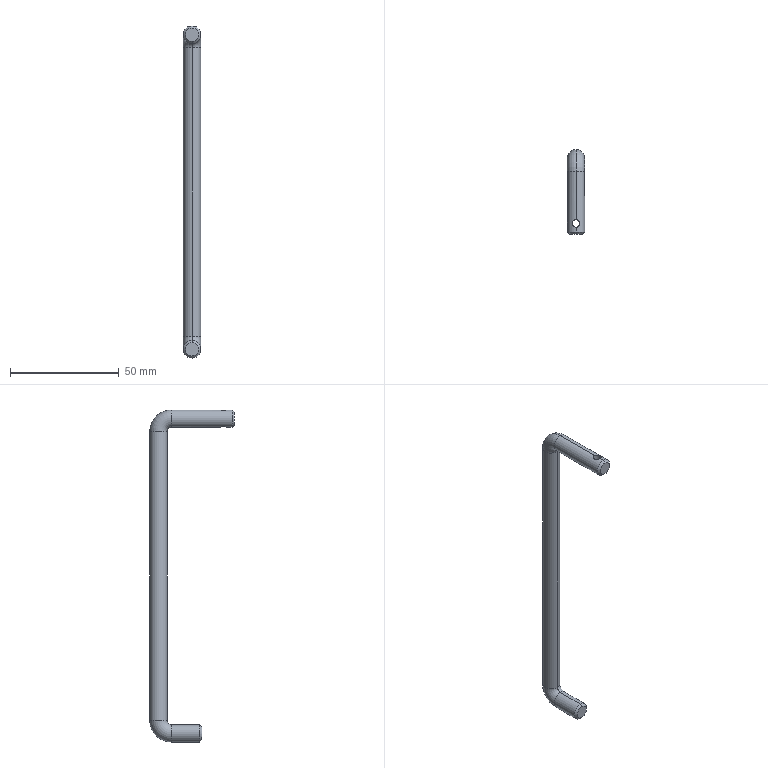Part | SolidWorks | features BaseBody 1 | 1 solid | 18 faces | box 8 x 39 x 153 mm | volume 9696 mm3 | cylinder 8 | cone 4 | torus 4 | plane 2 | commonest cylinder face diameters 8 x6 3.5 x2
STEP:
#1=CARTESIAN_POINT('',(1.75,-30.,76.097));
#2=VERTEX_POINT('',#1);
#3=CARTESIAN_POINT('',(1.75,-30.,68.903));
#4=VERTEX_POINT('',#3);
#5=CARTESIAN_POINT('',(1.75,-30.,132.));
#6=DIRECTION('',(0.,0.,-1.));
#7=VECTOR('',#6,1000.);
#8=LINE('',#5,#7);
#9=EDGE_CURVE('',#2,#4,#8,.T.);
#10=ORIENTED_EDGE('',*,*,#9,.F.);
#11=CARTESIAN_POINT('',(0.,-28.25,76.5));
#12=VERTEX_POINT('',#11);
#13=CARTESIAN_POINT('',(0.,-28.25,76.5));
#14=CARTESIAN_POINT('',(0.1167,-28.25,76.5));
#15=CARTESIAN_POINT('',(0.2317,-28.261,76.495));
#16=CARTESIAN_POINT('',(0.4573,-28.307,76.475));
#17=CARTESIAN_POINT('',(0.5697,-28.341,76.461));
#18=CARTESIAN_POINT('',(0.8889,-28.475,76.406));
#19=CARTESIAN_POINT('',(1.075,-28.6,76.357));
#20=CARTESIAN_POINT('',(1.321,-28.847,76.276));
#21=CARTESIAN_POINT('',(1.393,-28.935,76.25));
#22=CARTESIAN_POINT('',(1.487,-29.075,76.213));
#23=CARTESIAN_POINT('',(1.516,-29.124,76.202));
#24=CARTESIAN_POINT('',(1.569,-29.223,76.179));
#25=CARTESIAN_POINT('',(1.593,-29.272,76.169));
#26=CARTESIAN_POINT('',(1.706,-29.544,76.119));
#27=CARTESIAN_POINT('',(1.75,-29.768,76.097));
#28=CARTESIAN_POINT('',(1.75,-30.,76.097));
#29=B_SPLINE_CURVE_WITH_KNOTS('',3,(#13,#14,#15,#16,#17,#18,#19,#20,#21,#22,#23,#24,#25,#26,#27,#28),.UNSPECIFIED.,.F.,.F.,(4,2,2,2,2,2,2,4),(0.,0.125,0.25,0.5,0.625,0.6875,0.75,1.),.UNSPECIFIED.);
#30=EDGE_CURVE('',#12,#2,#29,.T.);
#31=ORIENTED_EDGE('',*,*,#30,.F.);
#32=CARTESIAN_POINT('',(-1.75,-30.,76.097));
#33=VERTEX_POINT('',#32);
#34=CARTESIAN_POINT('',(-1.75,-30.,76.097));
#35=CARTESIAN_POINT('',(-1.75,-29.884,76.097));
#36=CARTESIAN_POINT('',(-1.739,-29.769,76.102));
#37=CARTESIAN_POINT('',(-1.705,-29.6,76.118));
#38=CARTESIAN_POINT('',(-1.691,-29.545,76.125));
#39=CARTESIAN_POINT('',(-1.666,-29.462,76.137));
#40=CARTESIAN_POINT('',(-1.656,-29.434,76.141));
#41=CARTESIAN_POINT('',(-1.636,-29.379,76.15));
#42=CARTESIAN_POINT('',(-1.625,-29.351,76.155));
#43=CARTESIAN_POINT('',(-1.571,-29.22,76.179));
#44=CARTESIAN_POINT('',(-1.516,-29.118,76.202));
#45=CARTESIAN_POINT('',(-1.389,-28.93,76.252));
#46=CARTESIAN_POINT('',(-1.317,-28.842,76.278));
#47=CARTESIAN_POINT('',(-1.157,-28.683,76.33));
#48=CARTESIAN_POINT('',(-1.07,-28.611,76.355));
#49=CARTESIAN_POINT('',(-0.9274,-28.515,76.391));
#50=CARTESIAN_POINT('',(-0.8785,-28.486,76.403));
#51=CARTESIAN_POINT('',(-0.7783,-28.432,76.424));
#52=CARTESIAN_POINT('',(-0.7286,-28.408,76.433));
#53=CARTESIAN_POINT('',(-0.4588,-28.295,76.48));
#54=CARTESIAN_POINT('',(-0.233,-28.25,76.5));
#55=CARTESIAN_POINT('',(0.,-28.25,76.5));
#56=B_SPLINE_CURVE_WITH_KNOTS('',3,(#34,#35,#36,#37,#38,#39,#40,#41,#42,#43,#44,#45,#46,#47,#48,#49,#50,#51,#52,#53,#54,#55),.UNSPECIFIED.,.F.,.F.,(4,2,2,2,2,2,2,2,2,2,4),(0.,0.125,0.1875,0.2187,0.25,0.375,0.5,0.625,0.6875,0.75,1.),.UNSPECIFIED.);
#57=EDGE_CURVE('',#33,#12,#56,.T.);
#58=ORIENTED_EDGE('',*,*,#57,.F.);
#59=CARTESIAN_POINT('',(-1.75,-30.,68.903));
#60=VERTEX_POINT('',#59);
#61=CARTESIAN_POINT('',(-1.75,-30.,132.));
#62=DIRECTION('',(0.,0.,-1.));
#63=VECTOR('',#62,1000.);
#64=LINE('',#61,#63);
#65=EDGE_CURVE('',#33,#60,#64,.T.);
#66=ORIENTED_EDGE('',*,*,#65,.T.);
#67=CARTESIAN_POINT('',(0.,-28.25,68.5));
#68=VERTEX_POINT('',#67);
#69=CARTESIAN_POINT('',(0.,-28.25,68.5));
#70=CARTESIAN_POINT('',(-0.1167,-28.25,68.5));
#71=CARTESIAN_POINT('',(-0.2317,-28.261,68.505));
#72=CARTESIAN_POINT('',(-0.4008,-28.295,68.52));
#73=CARTESIAN_POINT('',(-0.4567,-28.309,68.526));
#74=CARTESIAN_POINT('',(-0.5672,-28.343,68.54));
#75=CARTESIAN_POINT('',(-0.6233,-28.364,68.549));
#76=CARTESIAN_POINT('',(-0.7812,-28.43,68.576));
#77=CARTESIAN_POINT('',(-0.8823,-28.485,68.597));
#78=CARTESIAN_POINT('',(-1.072,-28.612,68.645));
#79=CARTESIAN_POINT('',(-1.159,-28.684,68.671));
#80=CARTESIAN_POINT('',(-1.319,-28.844,68.723));
#81=CARTESIAN_POINT('',(-1.39,-28.93,68.748));
#82=CARTESIAN_POINT('',(-1.486,-29.074,68.786));
#83=CARTESIAN_POINT('',(-1.515,-29.123,68.798));
#84=CARTESIAN_POINT('',(-1.556,-29.198,68.815));
#85=CARTESIAN_POINT('',(-1.568,-29.223,68.82));
#86=CARTESIAN_POINT('',(-1.593,-29.274,68.831));
#87=CARTESIAN_POINT('',(-1.604,-29.299,68.836));
#88=CARTESIAN_POINT('',(-1.706,-29.543,68.881));
#89=CARTESIAN_POINT('',(-1.75,-29.768,68.903));
#90=CARTESIAN_POINT('',(-1.75,-30.,68.903));
#91=B_SPLINE_CURVE_WITH_KNOTS('',3,(#69,#70,#71,#72,#73,#74,#75,#76,#77,#78,#79,#80,#81,#82,#83,#84,#85,#86,#87,#88,#89,#90),.UNSPECIFIED.,.F.,.F.,(4,2,2,2,2,2,2,2,2,2,4),(0.,0.125,0.1875,0.25,0.375,0.5,0.625,0.6875,0.7187,0.75,1.),.UNSPECIFIED.);
#92=EDGE_CURVE('',#68,#60,#91,.T.);
#93=ORIENTED_EDGE('',*,*,#92,.F.);
#94=CARTESIAN_POINT('',(1.75,-30.,68.903));
#95=CARTESIAN_POINT('',(1.75,-29.77,68.903));
#96=CARTESIAN_POINT('',(1.703,-29.536,68.879));
#97=CARTESIAN_POINT('',(1.571,-29.221,68.821));
#98=CARTESIAN_POINT('',(1.518,-29.121,68.799));
#99=CARTESIAN_POINT('',(1.393,-28.934,68.75));
#100=CARTESIAN_POINT('',(1.319,-28.844,68.723));
#101=CARTESIAN_POINT('',(1.157,-28.682,68.67));
#102=CARTESIAN_POINT('',(1.069,-28.61,68.644));
#103=CARTESIAN_POINT('',(0.8816,-28.484,68.597));
#104=CARTESIAN_POINT('',(0.7831,-28.431,68.576));
#105=CARTESIAN_POINT('',(0.4592,-28.295,68.52));
#106=CARTESIAN_POINT('',(0.2331,-28.25,68.5));
#107=CARTESIAN_POINT('',(0.,-28.25,68.5));
#108=B_SPLINE_CURVE_WITH_KNOTS('',3,(#94,#95,#96,#97,#98,#99,#100,#101,#102,#103,#104,#105,#106,#107),.UNSPECIFIED.,.F.,.F.,(4,2,2,2,2,2,4),(0.,0.25,0.375,0.5,0.625,0.75,1.),.UNSPECIFIED.);
#109=EDGE_CURVE('',#4,#68,#108,.T.);
#110=ORIENTED_EDGE('',*,*,#109,.F.);
#111=EDGE_LOOP('',(#10,#31,#58,#66,#93,#110));
#112=FACE_OUTER_BOUND('',#111,.T.);
#113=CARTESIAN_POINT('',(0.,-30.,132.));
#114=DIRECTION('',(0.,0.,-1.));
#115=DIRECTION('',(-1.,0.,0.));
#116=AXIS2_PLACEMENT_3D('',#113,#114,#115);
#117=CYLINDRICAL_SURFACE('',#116,1.75);
#118=ADVANCED_FACE('',(#112),#117,.F.);
#119=CARTESIAN_POINT('',(0.,-35.,69.5));
#120=VERTEX_POINT('',#119);
#121=CARTESIAN_POINT('',(0.,-34.,68.5));
#122=VERTEX_POINT('',#121);
#123=CARTESIAN_POINT('',(0.,-35.,69.5));
#124=DIRECTION('',(0.,0.7071,-0.7071));
#125=VECTOR('',#124,1000.);
#126=LINE('',#123,#125);
#127=EDGE_CURVE('',#120,#122,#126,.T.);
#128=ORIENTED_EDGE('',*,*,#127,.F.);
#129=CARTESIAN_POINT('',(0.,-35.,75.5));
#130=VERTEX_POINT('',#129);
#131=CARTESIAN_POINT('',(0.,-35.,72.5));
#132=DIRECTION('',(0.,-1.,0.));
#133=DIRECTION('',(0.,0.,-1.));
#134=AXIS2_PLACEMENT_3D('',#131,#132,#133);
#135=CIRCLE('',#134,3.);
#136=EDGE_CURVE('',#130,#120,#135,.T.);
#137=ORIENTED_EDGE('',*,*,#136,.F.);
#138=CARTESIAN_POINT('',(0.,-34.,76.5));
#139=VERTEX_POINT('',#138);
#140=CARTESIAN_POINT('',(0.,-35.,75.5));
#141=DIRECTION('',(0.,0.7071,0.7071));
#142=VECTOR('',#141,1000.);
#143=LINE('',#140,#142);
#144=EDGE_CURVE('',#130,#139,#143,.T.);
#145=ORIENTED_EDGE('',*,*,#144,.T.);
#146=CARTESIAN_POINT('',(0.,-34.,72.5));
#147=DIRECTION('',(0.,1.,0.));
#148=DIRECTION('',(0.,0.,-1.));
#149=AXIS2_PLACEMENT_3D('',#146,#147,#148);
#150=CIRCLE('',#149,4.);
#151=EDGE_CURVE('',#122,#139,#150,.T.);
#152=ORIENTED_EDGE('',*,*,#151,.F.);
#153=EDGE_LOOP('',(#128,#137,#145,#152));
#154=FACE_OUTER_BOUND('',#153,.T.);
#155=CARTESIAN_POINT('',(0.,-35.,72.5));
#156=DIRECTION('',(0.,1.,0.));
#157=DIRECTION('',(0.,0.,1.));
#158=AXIS2_PLACEMENT_3D('',#155,#156,#157);
#159=CONICAL_SURFACE('',#158,3.,0.7854);
#160=ADVANCED_FACE('',(#154),#159,.T.);
#161=CARTESIAN_POINT('',(0.,-20.,-75.5));
#162=VERTEX_POINT('',#161);
#163=CARTESIAN_POINT('',(0.,-19.,-76.5));
#164=VERTEX_POINT('',#163);
#165=CARTESIAN_POINT('',(0.,-19.,-76.5));
#166=DIRECTION('',(0.,0.7071,-0.7071));
#167=VECTOR('',#166,1000.);
#168=LINE('',#165,#167);
#169=EDGE_CURVE('',#162,#164,#168,.T.);
#170=ORIENTED_EDGE('',*,*,#169,.F.);
#171=CARTESIAN_POINT('',(0.,-20.,-69.5));
#172=VERTEX_POINT('',#171);
#173=CARTESIAN_POINT('',(0.,-20.,-72.5));
#174=DIRECTION('',(0.,-1.,0.));
#175=DIRECTION('',(0.,0.,1.));
#176=AXIS2_PLACEMENT_3D('',#173,#174,#175);
#177=CIRCLE('',#176,3.);
#178=EDGE_CURVE('',#172,#162,#177,.T.);
#179=ORIENTED_EDGE('',*,*,#178,.F.);
#180=CARTESIAN_POINT('',(0.,-19.,-68.5));
#181=VERTEX_POINT('',#180);
#182=CARTESIAN_POINT('',(0.,-19.,-68.5));
#183=DIRECTION('',(0.,0.7071,0.7071));
#184=VECTOR('',#183,1000.);
#185=LINE('',#182,#184);
#186=EDGE_CURVE('',#172,#181,#185,.T.);
#187=ORIENTED_EDGE('',*,*,#186,.T.);
#188=CARTESIAN_POINT('',(0.,-19.,-72.5));
#189=DIRECTION('',(0.,1.,0.));
#190=DIRECTION('',(0.,0.,1.));
#191=AXIS2_PLACEMENT_3D('',#188,#189,#190);
#192=CIRCLE('',#191,4.);
#193=EDGE_CURVE('',#164,#181,#192,.T.);
#194=ORIENTED_EDGE('',*,*,#193,.F.);
#195=EDGE_LOOP('',(#170,#179,#187,#194));
#196=FACE_OUTER_BOUND('',#195,.T.);
#197=CARTESIAN_POINT('',(0.,-19.,-72.5));
#198=DIRECTION('',(0.,1.,0.));
#199=DIRECTION('',(0.,0.,1.));
#200=AXIS2_PLACEMENT_3D('',#197,#198,#199);
#201=CONICAL_SURFACE('',#200,4.,0.7854);
#202=ADVANCED_FACE('',(#196),#201,.T.);
#203=ORIENTED_EDGE('',*,*,#178,.T.);
#204=CARTESIAN_POINT('',(0.,-20.,-72.5));
#205=DIRECTION('',(0.,-1.,0.));
#206=DIRECTION('',(0.,0.,1.));
#207=AXIS2_PLACEMENT_3D('',#204,#205,#206);
#208=CIRCLE('',#207,3.);
#209=EDGE_CURVE('',#162,#172,#208,.T.);
#210=ORIENTED_EDGE('',*,*,#209,.T.);
#211=EDGE_LOOP('',(#203,#210));
#212=FACE_OUTER_BOUND('',#211,.T.);
#213=CARTESIAN_POINT('',(0.,-20.,-72.5));
#214=DIRECTION('',(0.,1.,0.));
#215=DIRECTION('',(0.,0.,-1.));
#216=AXIS2_PLACEMENT_3D('',#213,#214,#215);
#217=PLANE('',#216);
#218=ADVANCED_FACE('',(#212),#217,.F.);
#219=ORIENTED_EDGE('',*,*,#136,.T.);
#220=CARTESIAN_POINT('',(0.,-35.,72.5));
#221=DIRECTION('',(0.,-1.,0.));
#222=DIRECTION('',(0.,0.,-1.));
#223=AXIS2_PLACEMENT_3D('',#220,#221,#222);
#224=CIRCLE('',#223,3.);
#225=EDGE_CURVE('',#120,#130,#224,.T.);
#226=ORIENTED_EDGE('',*,*,#225,.T.);
#227=EDGE_LOOP('',(#219,#226));
#228=FACE_OUTER_BOUND('',#227,.T.);
#229=CARTESIAN_POINT('',(0.,-35.,72.5));
#230=DIRECTION('',(0.,-1.,0.));
#231=DIRECTION('',(0.,0.,-1.));
#232=AXIS2_PLACEMENT_3D('',#229,#230,#231);
#233=PLANE('',#232);
#234=ADVANCED_FACE('',(#228),#233,.T.);
#235=CARTESIAN_POINT('',(0.,-6.,-76.5));
#236=VERTEX_POINT('',#235);
#237=CARTESIAN_POINT('',(0.,-20.,-76.5));
#238=DIRECTION('',(0.,1.,0.));
#239=VECTOR('',#238,1000.);
#240=LINE('',#237,#239);
#241=EDGE_CURVE('',#164,#236,#240,.T.);
#242=ORIENTED_EDGE('',*,*,#241,.F.);
#243=ORIENTED_EDGE('',*,*,#193,.T.);
#244=CARTESIAN_POINT('',(0.,-6.,-68.5));
#245=VERTEX_POINT('',#244);
#246=CARTESIAN_POINT('',(0.,-20.,-68.5));
#247=DIRECTION('',(0.,1.,0.));
#248=VECTOR('',#247,1000.);
#249=LINE('',#246,#248);
#250=EDGE_CURVE('',#181,#245,#249,.T.);
#251=ORIENTED_EDGE('',*,*,#250,.T.);
#252=CARTESIAN_POINT('',(0.,-6.,-72.5));
#253=DIRECTION('',(0.,1.,0.));
#254=DIRECTION('',(1.,0.,0.));
#255=AXIS2_PLACEMENT_3D('',#252,#253,#254);
#256=CIRCLE('',#255,4.);
#257=EDGE_CURVE('',#236,#245,#256,.T.);
#258=ORIENTED_EDGE('',*,*,#257,.F.);
#259=EDGE_LOOP('',(#242,#243,#251,#258));
#260=FACE_OUTER_BOUND('',#259,.T.);
#261=CARTESIAN_POINT('',(0.,-20.,-72.5));
#262=DIRECTION('',(0.,1.,0.));
#263=DIRECTION('',(0.,0.,1.));
#264=AXIS2_PLACEMENT_3D('',#261,#262,#263);
#265=CYLINDRICAL_SURFACE('',#264,4.);
#266=ADVANCED_FACE('',(#260),#265,.T.);
#267=CARTESIAN_POINT('',(0.,4.,-66.5));
#268=VERTEX_POINT('',#267);
#269=CARTESIAN_POINT('',(0.,-6.,-66.5));
#270=DIRECTION('',(1.,0.,0.));
#271=DIRECTION('',(0.,0.,-1.));
#272=AXIS2_PLACEMENT_3D('',#269,#270,#271);
#273=CIRCLE('',#272,10.);
#274=EDGE_CURVE('',#236,#268,#273,.T.);
#275=ORIENTED_EDGE('',*,*,#274,.F.);
#276=ORIENTED_EDGE('',*,*,#257,.T.);
#277=CARTESIAN_POINT('',(0.,-4.,-66.5));
#278=VERTEX_POINT('',#277);
#279=CARTESIAN_POINT('',(0.,-6.,-66.5));
#280=DIRECTION('',(1.,0.,0.));
#281=DIRECTION('',(0.,0.,-1.));
#282=AXIS2_PLACEMENT_3D('',#279,#280,#281);
#283=CIRCLE('',#282,2.);
#284=EDGE_CURVE('',#245,#278,#283,.T.);
#285=ORIENTED_EDGE('',*,*,#284,.T.);
#286=CARTESIAN_POINT('',(0.,0.,-66.5));
#287=DIRECTION('',(0.,0.,1.));
#288=DIRECTION('',(1.,0.,0.));
#289=AXIS2_PLACEMENT_3D('',#286,#287,#288);
#290=CIRCLE('',#289,4.);
#291=EDGE_CURVE('',#268,#278,#290,.T.);
#292=ORIENTED_EDGE('',*,*,#291,.F.);
#293=EDGE_LOOP('',(#275,#276,#285,#292));
#294=FACE_OUTER_BOUND('',#293,.T.);
#295=CARTESIAN_POINT('',(0.,-6.,-66.5));
#296=DIRECTION('',(1.,0.,0.));
#297=DIRECTION('',(0.,0.,-1.));
#298=AXIS2_PLACEMENT_3D('',#295,#296,#297);
#299=TOROIDAL_SURFACE('',#298,6.,4.);
#300=ADVANCED_FACE('',(#294),#299,.T.);
#301=CARTESIAN_POINT('',(0.,4.,66.5));
#302=VERTEX_POINT('',#301);
#303=CARTESIAN_POINT('',(0.,4.,-66.5));
#304=DIRECTION('',(0.,0.,1.));
#305=VECTOR('',#304,1000.);
#306=LINE('',#303,#305);
#307=EDGE_CURVE('',#268,#302,#306,.T.);
#308=ORIENTED_EDGE('',*,*,#307,.F.);
#309=ORIENTED_EDGE('',*,*,#291,.T.);
#310=CARTESIAN_POINT('',(0.,-4.,66.5));
#311=VERTEX_POINT('',#310);
#312=CARTESIAN_POINT('',(0.,-4.,-66.5));
#313=DIRECTION('',(0.,0.,1.));
#314=VECTOR('',#313,1000.);
#315=LINE('',#312,#314);
#316=EDGE_CURVE('',#278,#311,#315,.T.);
#317=ORIENTED_EDGE('',*,*,#316,.T.);
#318=CARTESIAN_POINT('',(0.,0.,66.5));
#319=DIRECTION('',(0.,0.,1.));
#320=DIRECTION('',(1.,0.,0.));
#321=AXIS2_PLACEMENT_3D('',#318,#319,#320);
#322=CIRCLE('',#321,4.);
#323=EDGE_CURVE('',#302,#311,#322,.T.);
#324=ORIENTED_EDGE('',*,*,#323,.F.);
#325=EDGE_LOOP('',(#308,#309,#317,#324));
#326=FACE_OUTER_BOUND('',#325,.T.);
#327=CARTESIAN_POINT('',(0.,0.,-66.5));
#328=DIRECTION('',(0.,0.,1.));
#329=DIRECTION('',(0.,-1.,0.));
#330=AXIS2_PLACEMENT_3D('',#327,#328,#329);
#331=CYLINDRICAL_SURFACE('',#330,4.);
#332=ADVANCED_FACE('',(#326),#331,.T.);
#333=CARTESIAN_POINT('',(0.,-6.,76.5));
#334=VERTEX_POINT('',#333);
#335=CARTESIAN_POINT('',(0.,-6.,66.5));
#336=DIRECTION('',(1.,0.,0.));
#337=DIRECTION('',(0.,0.,-1.));
#338=AXIS2_PLACEMENT_3D('',#335,#336,#337);
#339=CIRCLE('',#338,10.);
#340=EDGE_CURVE('',#302,#334,#339,.T.);
#341=ORIENTED_EDGE('',*,*,#340,.F.);
#342=ORIENTED_EDGE('',*,*,#323,.T.);
#343=CARTESIAN_POINT('',(0.,-6.,68.5));
#344=VERTEX_POINT('',#343);
#345=CARTESIAN_POINT('',(0.,-6.,66.5));
#346=DIRECTION('',(1.,0.,0.));
#347=DIRECTION('',(0.,0.,-1.));
#348=AXIS2_PLACEMENT_3D('',#345,#346,#347);
#349=CIRCLE('',#348,2.);
#350=EDGE_CURVE('',#311,#344,#349,.T.);
#351=ORIENTED_EDGE('',*,*,#350,.T.);
#352=CARTESIAN_POINT('',(0.,-6.,72.5));
#353=DIRECTION('',(0.,-1.,0.));
#354=DIRECTION('',(1.,0.,0.));
#355=AXIS2_PLACEMENT_3D('',#352,#353,#354);
#356=CIRCLE('',#355,4.);
#357=EDGE_CURVE('',#334,#344,#356,.T.);
#358=ORIENTED_EDGE('',*,*,#357,.F.);
#359=EDGE_LOOP('',(#341,#342,#351,#358));
#360=FACE_OUTER_BOUND('',#359,.T.);
#361=CARTESIAN_POINT('',(0.,-6.,66.5));
#362=DIRECTION('',(1.,0.,0.));
#363=DIRECTION('',(0.,0.,-1.));
#364=AXIS2_PLACEMENT_3D('',#361,#362,#363);
#365=TOROIDAL_SURFACE('',#364,6.,4.);
#366=ADVANCED_FACE('',(#360),#365,.T.);
#367=CARTESIAN_POINT('',(0.,-6.,76.5));
#368=DIRECTION('',(0.,-1.,0.));
#369=VECTOR('',#368,1000.);
#370=LINE('',#367,#369);
#371=EDGE_CURVE('',#334,#12,#370,.T.);
#372=ORIENTED_EDGE('',*,*,#371,.F.);
#373=ORIENTED_EDGE('',*,*,#357,.T.);
#374=CARTESIAN_POINT('',(0.,-6.,68.5));
#375=DIRECTION('',(0.,-1.,0.));
#376=VECTOR('',#375,1000.);
#377=LINE('',#374,#376);
#378=EDGE_CURVE('',#344,#68,#377,.T.);
#379=ORIENTED_EDGE('',*,*,#378,.T.);
#380=ORIENTED_EDGE('',*,*,#92,.T.);
#381=CARTESIAN_POINT('',(0.,-31.75,68.5));
#382=VERTEX_POINT('',#381);
#383=CARTESIAN_POINT('',(-1.75,-30.,68.903));
#384=CARTESIAN_POINT('',(-1.75,-30.116,68.903));
#385=CARTESIAN_POINT('',(-1.739,-30.231,68.898));
#386=CARTESIAN_POINT('',(-1.705,-30.4,68.882));
#387=CARTESIAN_POINT('',(-1.691,-30.455,68.875));
#388=CARTESIAN_POINT('',(-1.657,-30.566,68.859));
#389=CARTESIAN_POINT('',(-1.636,-30.623,68.85));
#390=CARTESIAN_POINT('',(-1.57,-30.781,68.821));
#391=CARTESIAN_POINT('',(-1.517,-30.88,68.798));
#392=CARTESIAN_POINT('',(-1.392,-31.068,68.749));
#393=CARTESIAN_POINT('',(-1.318,-31.157,68.722));
#394=CARTESIAN_POINT('',(-1.155,-31.319,68.67));
#395=CARTESIAN_POINT('',(-1.068,-31.391,68.644));
#396=CARTESIAN_POINT('',(-0.8804,-31.517,68.597));
#397=CARTESIAN_POINT('',(-0.7819,-31.57,68.576));
#398=CARTESIAN_POINT('',(-0.4584,-31.705,68.52));
#399=CARTESIAN_POINT('',(-0.2328,-31.75,68.5));
#400=CARTESIAN_POINT('',(0.,-31.75,68.5));
#401=B_SPLINE_CURVE_WITH_KNOTS('',3,(#383,#384,#385,#386,#387,#388,#389,#390,#391,#392,#393,#394,#395,#396,#397,#398,#399,#400),.UNSPECIFIED.,.F.,.F.,(4,2,2,2,2,2,2,2,4),(0.,0.125,0.1875,0.25,0.375,0.5,0.625,0.75,1.),.UNSPECIFIED.);
#402=EDGE_CURVE('',#60,#382,#401,.T.);
#403=ORIENTED_EDGE('',*,*,#402,.T.);
#404=CARTESIAN_POINT('',(0.,-6.,68.5));
#405=DIRECTION('',(0.,-1.,0.));
#406=VECTOR('',#405,1000.);
#407=LINE('',#404,#406);
#408=EDGE_CURVE('',#382,#122,#407,.T.);
#409=ORIENTED_EDGE('',*,*,#408,.T.);
#410=ORIENTED_EDGE('',*,*,#151,.T.);
#411=CARTESIAN_POINT('',(0.,-31.75,76.5));
#412=VERTEX_POINT('',#411);
#413=CARTESIAN_POINT('',(0.,-6.,76.5));
#414=DIRECTION('',(0.,-1.,0.));
#415=VECTOR('',#414,1000.);
#416=LINE('',#413,#415);
#417=EDGE_CURVE('',#412,#139,#416,.T.);
#418=ORIENTED_EDGE('',*,*,#417,.F.);
#419=CARTESIAN_POINT('',(0.,-31.75,76.5));
#420=CARTESIAN_POINT('',(-0.1165,-31.75,76.5));
#421=CARTESIAN_POINT('',(-0.2312,-31.739,76.495));
#422=CARTESIAN_POINT('',(-0.4563,-31.694,76.475));
#423=CARTESIAN_POINT('',(-0.5683,-31.659,76.461));
#424=CARTESIAN_POINT('',(-0.7811,-31.57,76.424));
#425=CARTESIAN_POINT('',(-0.8813,-31.517,76.403));
#426=CARTESIAN_POINT('',(-1.069,-31.391,76.356));
#427=CARTESIAN_POINT('',(-1.156,-31.319,76.33));
#428=CARTESIAN_POINT('',(-1.32,-31.155,76.277));
#429=CARTESIAN_POINT('',(-1.393,-31.066,76.25));
#430=CARTESIAN_POINT('',(-1.486,-30.926,76.214));
#431=CARTESIAN_POINT('',(-1.515,-30.878,76.202));
#432=CARTESIAN_POINT('',(-1.569,-30.778,76.18));
#433=CARTESIAN_POINT('',(-1.592,-30.729,76.17));
#434=CARTESIAN_POINT('',(-1.706,-30.457,76.119));
#435=CARTESIAN_POINT('',(-1.75,-30.232,76.097));
#436=CARTESIAN_POINT('',(-1.75,-30.,76.097));
#437=B_SPLINE_CURVE_WITH_KNOTS('',3,(#419,#420,#421,#422,#423,#424,#425,#426,#427,#428,#429,#430,#431,#432,#433,#434,#435,#436),.UNSPECIFIED.,.F.,.F.,(4,2,2,2,2,2,2,2,4),(0.,0.125,0.25,0.375,0.5,0.625,0.6875,0.75,1.),.UNSPECIFIED.);
#438=EDGE_CURVE('',#412,#33,#437,.T.);
#439=ORIENTED_EDGE('',*,*,#438,.T.);
#440=ORIENTED_EDGE('',*,*,#57,.T.);
#441=EDGE_LOOP('',(#372,#373,#379,#380,#403,#409,#410,#418,#439,#440));
#442=FACE_OUTER_BOUND('',#441,.T.);
#443=CARTESIAN_POINT('',(0.,-6.,72.5));
#444=DIRECTION('',(0.,-1.,0.));
#445=DIRECTION('',(0.,0.,-1.));
#446=AXIS2_PLACEMENT_3D('',#443,#444,#445);
#447=CYLINDRICAL_SURFACE('',#446,4.);
#448=ADVANCED_FACE('',(#442),#447,.T.);
#449=CARTESIAN_POINT('',(0.,-6.,72.5));
#450=DIRECTION('',(0.,-1.,0.));
#451=DIRECTION('',(1.,0.,0.));
#452=AXIS2_PLACEMENT_3D('',#449,#450,#451);
#453=CIRCLE('',#452,4.);
#454=EDGE_CURVE('',#344,#334,#453,.T.);
#455=ORIENTED_EDGE('',*,*,#454,.T.);
#456=ORIENTED_EDGE('',*,*,#371,.T.);
#457=ORIENTED_EDGE('',*,*,#30,.T.);
#458=CARTESIAN_POINT('',(1.75,-30.,76.097));
#459=CARTESIAN_POINT('',(1.75,-30.116,76.097));
#460=CARTESIAN_POINT('',(1.739,-30.23,76.102));
#461=CARTESIAN_POINT('',(1.705,-30.399,76.118));
#462=CARTESIAN_POINT('',(1.691,-30.455,76.125));
#463=CARTESIAN_POINT('',(1.657,-30.565,76.141));
#464=CARTESIAN_POINT('',(1.637,-30.622,76.15));
#465=CARTESIAN_POINT('',(1.571,-30.78,76.179));
#466=CARTESIAN_POINT('',(1.518,-30.88,76.202));
#467=CARTESIAN_POINT('',(1.392,-31.067,76.251));
#468=CARTESIAN_POINT('',(1.318,-31.157,76.277));
#469=CARTESIAN_POINT('',(1.156,-31.319,76.33));
#470=CARTESIAN_POINT('',(1.068,-31.391,76.356));
#471=CARTESIAN_POINT('',(0.8805,-31.517,76.403));
#472=CARTESIAN_POINT('',(0.782,-31.57,76.424));
#473=CARTESIAN_POINT('',(0.4585,-31.705,76.48));
#474=CARTESIAN_POINT('',(0.2328,-31.75,76.5));
#475=CARTESIAN_POINT('',(0.,-31.75,76.5));
#476=B_SPLINE_CURVE_WITH_KNOTS('',3,(#458,#459,#460,#461,#462,#463,#464,#465,#466,#467,#468,#469,#470,#471,#472,#473,#474,#475),.UNSPECIFIED.,.F.,.F.,(4,2,2,2,2,2,2,2,4),(0.,0.125,0.1875,0.25,0.375,0.5,0.625,0.75,1.),.UNSPECIFIED.);
#477=EDGE_CURVE('',#2,#412,#476,.T.);
#478=ORIENTED_EDGE('',*,*,#477,.T.);
#479=ORIENTED_EDGE('',*,*,#417,.T.);
#480=CARTESIAN_POINT('',(0.,-34.,72.5));
#481=DIRECTION('',(0.,1.,0.));
#482=DIRECTION('',(0.,0.,-1.));
#483=AXIS2_PLACEMENT_3D('',#480,#481,#482);
#484=CIRCLE('',#483,4.);
#485=EDGE_CURVE('',#139,#122,#484,.T.);
#486=ORIENTED_EDGE('',*,*,#485,.T.);
#487=ORIENTED_EDGE('',*,*,#408,.F.);
#488=CARTESIAN_POINT('',(0.,-31.75,68.5));
#489=CARTESIAN_POINT('',(0.1166,-31.75,68.5));
#490=CARTESIAN_POINT('',(0.2314,-31.739,68.505));
#491=CARTESIAN_POINT('',(0.4567,-31.694,68.525));
#492=CARTESIAN_POINT('',(0.5687,-31.659,68.539));
#493=CARTESIAN_POINT('',(0.8883,-31.525,68.594));
#494=CARTESIAN_POINT('',(1.075,-31.401,68.643));
#495=CARTESIAN_POINT('',(1.321,-31.154,68.723));
#496=CARTESIAN_POINT('',(1.393,-31.066,68.75));
#497=CARTESIAN_POINT('',(1.487,-30.925,68.787));
#498=CARTESIAN_POINT('',(1.516,-30.877,68.798));
#499=CARTESIAN_POINT('',(1.569,-30.777,68.82));
#500=CARTESIAN_POINT('',(1.593,-30.728,68.831));
#501=CARTESIAN_POINT('',(1.706,-30.456,68.881));
#502=CARTESIAN_POINT('',(1.75,-30.232,68.903));
#503=CARTESIAN_POINT('',(1.75,-30.,68.903));
#504=B_SPLINE_CURVE_WITH_KNOTS('',3,(#488,#489,#490,#491,#492,#493,#494,#495,#496,#497,#498,#499,#500,#501,#502,#503),.UNSPECIFIED.,.F.,.F.,(4,2,2,2,2,2,2,4),(0.,0.125,0.25,0.5,0.625,0.6875,0.75,1.),.UNSPECIFIED.);
#505=EDGE_CURVE('',#382,#4,#504,.T.);
#506=ORIENTED_EDGE('',*,*,#505,.T.);
#507=ORIENTED_EDGE('',*,*,#109,.T.);
#508=ORIENTED_EDGE('',*,*,#378,.F.);
#509=EDGE_LOOP('',(#455,#456,#457,#478,#479,#486,#487,#506,#507,#508));
#510=FACE_OUTER_BOUND('',#509,.T.);
#511=CARTESIAN_POINT('',(0.,-6.,72.5));
#512=DIRECTION('',(0.,-1.,0.));
#513=DIRECTION('',(0.,0.,-1.));
#514=AXIS2_PLACEMENT_3D('',#511,#512,#513);
#515=CYLINDRICAL_SURFACE('',#514,4.);
#516=ADVANCED_FACE('',(#510),#515,.T.);
#517=CARTESIAN_POINT('',(0.,-19.,-72.5));
#518=DIRECTION('',(0.,1.,0.));
#519=DIRECTION('',(0.,0.,1.));
#520=AXIS2_PLACEMENT_3D('',#517,#518,#519);
#521=CIRCLE('',#520,4.);
#522=EDGE_CURVE('',#181,#164,#521,.T.);
#523=ORIENTED_EDGE('',*,*,#522,.T.);
#524=ORIENTED_EDGE('',*,*,#241,.T.);
#525=CARTESIAN_POINT('',(0.,-6.,-72.5));
#526=DIRECTION('',(0.,1.,0.));
#527=DIRECTION('',(1.,0.,0.));
#528=AXIS2_PLACEMENT_3D('',#525,#526,#527);
#529=CIRCLE('',#528,4.);
#530=EDGE_CURVE('',#245,#236,#529,.T.);
#531=ORIENTED_EDGE('',*,*,#530,.F.);
#532=ORIENTED_EDGE('',*,*,#250,.F.);
#533=EDGE_LOOP('',(#523,#524,#531,#532));
#534=FACE_OUTER_BOUND('',#533,.T.);
#535=CARTESIAN_POINT('',(0.,-20.,-72.5));
#536=DIRECTION('',(0.,1.,0.));
#537=DIRECTION('',(0.,0.,1.));
#538=AXIS2_PLACEMENT_3D('',#535,#536,#537);
#539=CYLINDRICAL_SURFACE('',#538,4.);
#540=ADVANCED_FACE('',(#534),#539,.T.);
#541=CARTESIAN_POINT('',(0.,0.,-66.5));
#542=DIRECTION('',(0.,0.,1.));
#543=DIRECTION('',(1.,0.,0.));
#544=AXIS2_PLACEMENT_3D('',#541,#542,#543);
#545=CIRCLE('',#544,4.);
#546=EDGE_CURVE('',#278,#268,#545,.T.);
#547=ORIENTED_EDGE('',*,*,#546,.T.);
#548=ORIENTED_EDGE('',*,*,#307,.T.);
#549=CARTESIAN_POINT('',(0.,0.,66.5));
#550=DIRECTION('',(0.,0.,1.));
#551=DIRECTION('',(1.,0.,0.));
#552=AXIS2_PLACEMENT_3D('',#549,#550,#551);
#553=CIRCLE('',#552,4.);
#554=EDGE_CURVE('',#311,#302,#553,.T.);
#555=ORIENTED_EDGE('',*,*,#554,.F.);
#556=ORIENTED_EDGE('',*,*,#316,.F.);
#557=EDGE_LOOP('',(#547,#548,#555,#556));
#558=FACE_OUTER_BOUND('',#557,.T.);
#559=CARTESIAN_POINT('',(0.,0.,-66.5));
#560=DIRECTION('',(0.,0.,1.));
#561=DIRECTION('',(0.,-1.,0.));
#562=AXIS2_PLACEMENT_3D('',#559,#560,#561);
#563=CYLINDRICAL_SURFACE('',#562,4.);
#564=ADVANCED_FACE('',(#558),#563,.T.);
#565=ORIENTED_EDGE('',*,*,#209,.F.);
#566=ORIENTED_EDGE('',*,*,#169,.T.);
#567=ORIENTED_EDGE('',*,*,#522,.F.);
#568=ORIENTED_EDGE('',*,*,#186,.F.);
#569=EDGE_LOOP('',(#565,#566,#567,#568));
#570=FACE_OUTER_BOUND('',#569,.T.);
#571=CARTESIAN_POINT('',(0.,-19.,-72.5));
#572=DIRECTION('',(0.,1.,0.));
#573=DIRECTION('',(0.,0.,1.));
#574=AXIS2_PLACEMENT_3D('',#571,#572,#573);
#575=CONICAL_SURFACE('',#574,4.,0.7854);
#576=ADVANCED_FACE('',(#570),#575,.T.);
#577=ORIENTED_EDGE('',*,*,#225,.F.);
#578=ORIENTED_EDGE('',*,*,#127,.T.);
#579=ORIENTED_EDGE('',*,*,#485,.F.);
#580=ORIENTED_EDGE('',*,*,#144,.F.);
#581=EDGE_LOOP('',(#577,#578,#579,#580));
#582=FACE_OUTER_BOUND('',#581,.T.);
#583=CARTESIAN_POINT('',(0.,-35.,72.5));
#584=DIRECTION('',(0.,1.,0.));
#585=DIRECTION('',(0.,0.,1.));
#586=AXIS2_PLACEMENT_3D('',#583,#584,#585);
#587=CONICAL_SURFACE('',#586,3.,0.7854);
#588=ADVANCED_FACE('',(#582),#587,.T.);
#589=ORIENTED_EDGE('',*,*,#477,.F.);
#590=ORIENTED_EDGE('',*,*,#9,.T.);
#591=ORIENTED_EDGE('',*,*,#505,.F.);
#592=ORIENTED_EDGE('',*,*,#402,.F.);
#593=ORIENTED_EDGE('',*,*,#65,.F.);
#594=ORIENTED_EDGE('',*,*,#438,.F.);
#595=EDGE_LOOP('',(#589,#590,#591,#592,#593,#594));
#596=FACE_OUTER_BOUND('',#595,.T.);
#597=CARTESIAN_POINT('',(0.,-30.,132.));
#598=DIRECTION('',(0.,0.,-1.));
#599=DIRECTION('',(-1.,0.,0.));
#600=AXIS2_PLACEMENT_3D('',#597,#598,#599);
#601=CYLINDRICAL_SURFACE('',#600,1.75);
#602=ADVANCED_FACE('',(#596),#601,.F.);
#603=ORIENTED_EDGE('',*,*,#530,.T.);
#604=ORIENTED_EDGE('',*,*,#274,.T.);
#605=ORIENTED_EDGE('',*,*,#546,.F.);
#606=ORIENTED_EDGE('',*,*,#284,.F.);
#607=EDGE_LOOP('',(#603,#604,#605,#606));
#608=FACE_OUTER_BOUND('',#607,.T.);
#609=CARTESIAN_POINT('',(0.,-6.,-66.5));
#610=DIRECTION('',(1.,0.,0.));
#611=DIRECTION('',(0.,0.,-1.));
#612=AXIS2_PLACEMENT_3D('',#609,#610,#611);
#613=TOROIDAL_SURFACE('',#612,6.,4.);
#614=ADVANCED_FACE('',(#608),#613,.T.);
#615=ORIENTED_EDGE('',*,*,#554,.T.);
#616=ORIENTED_EDGE('',*,*,#340,.T.);
#617=ORIENTED_EDGE('',*,*,#454,.F.);
#618=ORIENTED_EDGE('',*,*,#350,.F.);
#619=EDGE_LOOP('',(#615,#616,#617,#618));
#620=FACE_OUTER_BOUND('',#619,.T.);
#621=CARTESIAN_POINT('',(0.,-6.,66.5));
#622=DIRECTION('',(1.,0.,0.));
#623=DIRECTION('',(0.,0.,-1.));
#624=AXIS2_PLACEMENT_3D('',#621,#622,#623);
#625=TOROIDAL_SURFACE('',#624,6.,4.);
#626=ADVANCED_FACE('',(#620),#625,.T.);
#627=CLOSED_SHELL('',(#118,#160,#202,#218,#234,#266,#300,#332,#366,#448,#516,#540,#564,#576,#588,#602,#614,#626));
#628=MANIFOLD_SOLID_BREP('',#627);
#629=CARTESIAN_POINT('',(0.,0.,0.));
#630=DIRECTION('',(0.,0.,1.));
#631=DIRECTION('',(1.,0.,0.));
#632=AXIS2_PLACEMENT_3D('',#629,#630,#631);
#633=(LENGTH_UNIT()NAMED_UNIT(*)SI_UNIT(.MILLI.,.METRE.));
#634=UNCERTAINTY_MEASURE_WITH_UNIT(LENGTH_MEASURE(0.00001),#633,'','');
#635=(NAMED_UNIT(*)PLANE_ANGLE_UNIT()SI_UNIT($,.RADIAN.));
#636=(NAMED_UNIT(*)SI_UNIT($,.STERADIAN.)SOLID_ANGLE_UNIT());
#637=(GEOMETRIC_REPRESENTATION_CONTEXT(3)GLOBAL_UNCERTAINTY_ASSIGNED_CONTEXT((#634))GLOBAL_UNIT_ASSIGNED_CONTEXT((#633,#635,#636))REPRESENTATION_CONTEXT('',''));
#638=ADVANCED_BREP_SHAPE_REPRESENTATION('',(#628,#632),#637);